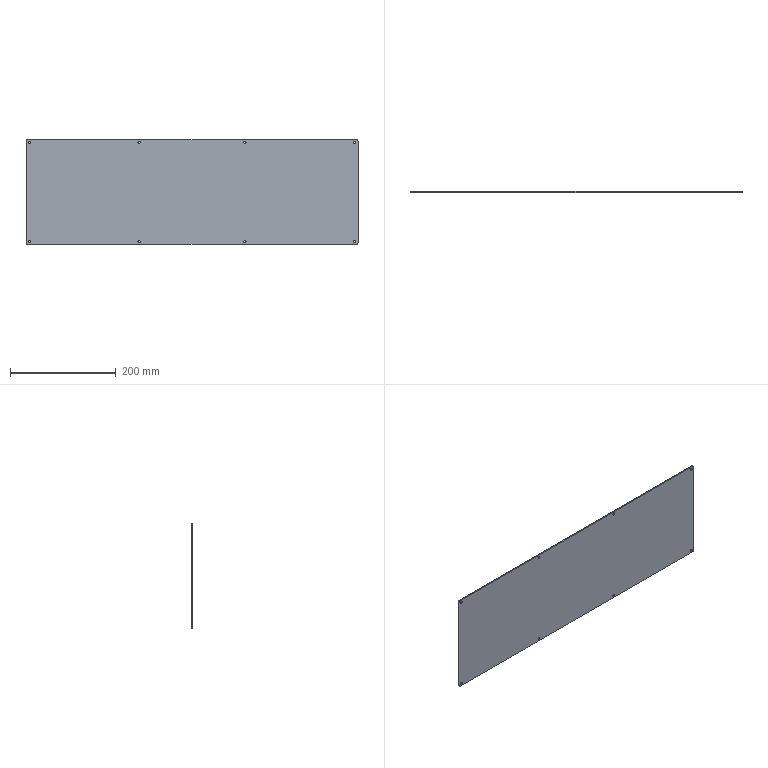Part | SolidWorks | features BaseBody 1 | 1 solid | 26 faces | box 628 x 2 x 198 mm | volume 248418 mm3 | cylinder 20 | plane 6 | commonest cylinder face diameters 4.5 x16 6 x4
STEP:
#1=CARTESIAN_POINT('',(307.5,0.,91.75));
#2=VERTEX_POINT('',#1);
#3=CARTESIAN_POINT('',(307.5,2.,91.75));
#4=VERTEX_POINT('',#3);
#5=CARTESIAN_POINT('',(307.5,-0.001,91.75));
#6=DIRECTION('',(0.,1.,0.));
#7=VECTOR('',#6,1000.);
#8=LINE('',#5,#7);
#9=EDGE_CURVE('',#2,#4,#8,.T.);
#10=ORIENTED_EDGE('',*,*,#9,.F.);
#11=CARTESIAN_POINT('',(307.5,0.,96.25));
#12=VERTEX_POINT('',#11);
#13=CARTESIAN_POINT('',(307.5,0.,94.));
#14=DIRECTION('',(0.,-1.,0.));
#15=DIRECTION('',(0.,0.,1.));
#16=AXIS2_PLACEMENT_3D('',#13,#14,#15);
#17=CIRCLE('',#16,2.25);
#18=EDGE_CURVE('',#2,#12,#17,.T.);
#19=ORIENTED_EDGE('',*,*,#18,.T.);
#20=CARTESIAN_POINT('',(307.5,2.,96.25));
#21=VERTEX_POINT('',#20);
#22=CARTESIAN_POINT('',(307.5,-0.001,96.25));
#23=DIRECTION('',(0.,1.,0.));
#24=VECTOR('',#23,1000.);
#25=LINE('',#22,#24);
#26=EDGE_CURVE('',#12,#21,#25,.T.);
#27=ORIENTED_EDGE('',*,*,#26,.T.);
#28=CARTESIAN_POINT('',(307.5,2.,94.));
#29=DIRECTION('',(0.,1.,0.));
#30=DIRECTION('',(0.,0.,1.));
#31=AXIS2_PLACEMENT_3D('',#28,#29,#30);
#32=CIRCLE('',#31,2.25);
#33=EDGE_CURVE('',#21,#4,#32,.T.);
#34=ORIENTED_EDGE('',*,*,#33,.T.);
#35=EDGE_LOOP('',(#10,#19,#27,#34));
#36=FACE_OUTER_BOUND('',#35,.T.);
#37=CARTESIAN_POINT('',(307.5,-0.001,94.));
#38=DIRECTION('',(0.,1.,0.));
#39=DIRECTION('',(0.,0.,1.));
#40=AXIS2_PLACEMENT_3D('',#37,#38,#39);
#41=CYLINDRICAL_SURFACE('',#40,2.25);
#42=ADVANCED_FACE('',(#36),#41,.F.);
#43=CARTESIAN_POINT('',(-307.5,0.,91.75));
#44=VERTEX_POINT('',#43);
#45=CARTESIAN_POINT('',(-307.5,2.,91.75));
#46=VERTEX_POINT('',#45);
#47=CARTESIAN_POINT('',(-307.5,-0.001,91.75));
#48=DIRECTION('',(0.,1.,0.));
#49=VECTOR('',#48,1000.);
#50=LINE('',#47,#49);
#51=EDGE_CURVE('',#44,#46,#50,.T.);
#52=ORIENTED_EDGE('',*,*,#51,.F.);
#53=CARTESIAN_POINT('',(-307.5,0.,96.25));
#54=VERTEX_POINT('',#53);
#55=CARTESIAN_POINT('',(-307.5,0.,94.));
#56=DIRECTION('',(0.,-1.,0.));
#57=DIRECTION('',(0.,0.,1.));
#58=AXIS2_PLACEMENT_3D('',#55,#56,#57);
#59=CIRCLE('',#58,2.25);
#60=EDGE_CURVE('',#44,#54,#59,.T.);
#61=ORIENTED_EDGE('',*,*,#60,.T.);
#62=CARTESIAN_POINT('',(-307.5,2.,96.25));
#63=VERTEX_POINT('',#62);
#64=CARTESIAN_POINT('',(-307.5,-0.001,96.25));
#65=DIRECTION('',(0.,1.,0.));
#66=VECTOR('',#65,1000.);
#67=LINE('',#64,#66);
#68=EDGE_CURVE('',#54,#63,#67,.T.);
#69=ORIENTED_EDGE('',*,*,#68,.T.);
#70=CARTESIAN_POINT('',(-307.5,2.,94.));
#71=DIRECTION('',(0.,1.,0.));
#72=DIRECTION('',(0.,0.,-1.));
#73=AXIS2_PLACEMENT_3D('',#70,#71,#72);
#74=CIRCLE('',#73,2.25);
#75=EDGE_CURVE('',#63,#46,#74,.T.);
#76=ORIENTED_EDGE('',*,*,#75,.T.);
#77=EDGE_LOOP('',(#52,#61,#69,#76));
#78=FACE_OUTER_BOUND('',#77,.T.);
#79=CARTESIAN_POINT('',(-307.5,-0.001,94.));
#80=DIRECTION('',(0.,1.,0.));
#81=DIRECTION('',(0.,0.,1.));
#82=AXIS2_PLACEMENT_3D('',#79,#80,#81);
#83=CYLINDRICAL_SURFACE('',#82,2.25);
#84=ADVANCED_FACE('',(#78),#83,.F.);
#85=CARTESIAN_POINT('',(-100.,0.,91.75));
#86=VERTEX_POINT('',#85);
#87=CARTESIAN_POINT('',(-100.,2.,91.75));
#88=VERTEX_POINT('',#87);
#89=CARTESIAN_POINT('',(-100.,-0.001,91.75));
#90=DIRECTION('',(0.,1.,0.));
#91=VECTOR('',#90,1000.);
#92=LINE('',#89,#91);
#93=EDGE_CURVE('',#86,#88,#92,.T.);
#94=ORIENTED_EDGE('',*,*,#93,.F.);
#95=CARTESIAN_POINT('',(-100.,0.,96.25));
#96=VERTEX_POINT('',#95);
#97=CARTESIAN_POINT('',(-100.,0.,94.));
#98=DIRECTION('',(0.,-1.,0.));
#99=DIRECTION('',(0.,0.,1.));
#100=AXIS2_PLACEMENT_3D('',#97,#98,#99);
#101=CIRCLE('',#100,2.25);
#102=EDGE_CURVE('',#86,#96,#101,.T.);
#103=ORIENTED_EDGE('',*,*,#102,.T.);
#104=CARTESIAN_POINT('',(-100.,2.,96.25));
#105=VERTEX_POINT('',#104);
#106=CARTESIAN_POINT('',(-100.,-0.001,96.25));
#107=DIRECTION('',(0.,1.,0.));
#108=VECTOR('',#107,1000.);
#109=LINE('',#106,#108);
#110=EDGE_CURVE('',#96,#105,#109,.T.);
#111=ORIENTED_EDGE('',*,*,#110,.T.);
#112=CARTESIAN_POINT('',(-100.,2.,94.));
#113=DIRECTION('',(0.,1.,0.));
#114=DIRECTION('',(0.,0.,-1.));
#115=AXIS2_PLACEMENT_3D('',#112,#113,#114);
#116=CIRCLE('',#115,2.25);
#117=EDGE_CURVE('',#105,#88,#116,.T.);
#118=ORIENTED_EDGE('',*,*,#117,.T.);
#119=EDGE_LOOP('',(#94,#103,#111,#118));
#120=FACE_OUTER_BOUND('',#119,.T.);
#121=CARTESIAN_POINT('',(-100.,-0.001,94.));
#122=DIRECTION('',(0.,1.,0.));
#123=DIRECTION('',(0.,0.,1.));
#124=AXIS2_PLACEMENT_3D('',#121,#122,#123);
#125=CYLINDRICAL_SURFACE('',#124,2.25);
#126=ADVANCED_FACE('',(#120),#125,.F.);
#127=CARTESIAN_POINT('',(-100.,0.,-96.25));
#128=VERTEX_POINT('',#127);
#129=CARTESIAN_POINT('',(-100.,2.,-96.25));
#130=VERTEX_POINT('',#129);
#131=CARTESIAN_POINT('',(-100.,-0.001,-96.25));
#132=DIRECTION('',(0.,1.,0.));
#133=VECTOR('',#132,1000.);
#134=LINE('',#131,#133);
#135=EDGE_CURVE('',#128,#130,#134,.T.);
#136=ORIENTED_EDGE('',*,*,#135,.F.);
#137=CARTESIAN_POINT('',(-100.,0.,-91.75));
#138=VERTEX_POINT('',#137);
#139=CARTESIAN_POINT('',(-100.,0.,-94.));
#140=DIRECTION('',(0.,-1.,0.));
#141=DIRECTION('',(0.,0.,1.));
#142=AXIS2_PLACEMENT_3D('',#139,#140,#141);
#143=CIRCLE('',#142,2.25);
#144=EDGE_CURVE('',#128,#138,#143,.T.);
#145=ORIENTED_EDGE('',*,*,#144,.T.);
#146=CARTESIAN_POINT('',(-100.,2.,-91.75));
#147=VERTEX_POINT('',#146);
#148=CARTESIAN_POINT('',(-100.,-0.001,-91.75));
#149=DIRECTION('',(0.,1.,0.));
#150=VECTOR('',#149,1000.);
#151=LINE('',#148,#150);
#152=EDGE_CURVE('',#138,#147,#151,.T.);
#153=ORIENTED_EDGE('',*,*,#152,.T.);
#154=CARTESIAN_POINT('',(-100.,2.,-94.));
#155=DIRECTION('',(0.,1.,0.));
#156=DIRECTION('',(0.,0.,1.));
#157=AXIS2_PLACEMENT_3D('',#154,#155,#156);
#158=CIRCLE('',#157,2.25);
#159=EDGE_CURVE('',#147,#130,#158,.T.);
#160=ORIENTED_EDGE('',*,*,#159,.T.);
#161=EDGE_LOOP('',(#136,#145,#153,#160));
#162=FACE_OUTER_BOUND('',#161,.T.);
#163=CARTESIAN_POINT('',(-100.,-0.001,-94.));
#164=DIRECTION('',(0.,1.,0.));
#165=DIRECTION('',(0.,0.,1.));
#166=AXIS2_PLACEMENT_3D('',#163,#164,#165);
#167=CYLINDRICAL_SURFACE('',#166,2.25);
#168=ADVANCED_FACE('',(#162),#167,.F.);
#169=CARTESIAN_POINT('',(100.,0.,91.75));
#170=VERTEX_POINT('',#169);
#171=CARTESIAN_POINT('',(100.,2.,91.75));
#172=VERTEX_POINT('',#171);
#173=CARTESIAN_POINT('',(100.,-0.001,91.75));
#174=DIRECTION('',(0.,1.,0.));
#175=VECTOR('',#174,1000.);
#176=LINE('',#173,#175);
#177=EDGE_CURVE('',#170,#172,#176,.T.);
#178=ORIENTED_EDGE('',*,*,#177,.F.);
#179=CARTESIAN_POINT('',(100.,0.,96.25));
#180=VERTEX_POINT('',#179);
#181=CARTESIAN_POINT('',(100.,0.,94.));
#182=DIRECTION('',(0.,-1.,0.));
#183=DIRECTION('',(0.,0.,1.));
#184=AXIS2_PLACEMENT_3D('',#181,#182,#183);
#185=CIRCLE('',#184,2.25);
#186=EDGE_CURVE('',#170,#180,#185,.T.);
#187=ORIENTED_EDGE('',*,*,#186,.T.);
#188=CARTESIAN_POINT('',(100.,2.,96.25));
#189=VERTEX_POINT('',#188);
#190=CARTESIAN_POINT('',(100.,-0.001,96.25));
#191=DIRECTION('',(0.,1.,0.));
#192=VECTOR('',#191,1000.);
#193=LINE('',#190,#192);
#194=EDGE_CURVE('',#180,#189,#193,.T.);
#195=ORIENTED_EDGE('',*,*,#194,.T.);
#196=CARTESIAN_POINT('',(100.,2.,94.));
#197=DIRECTION('',(0.,1.,0.));
#198=DIRECTION('',(0.,0.,1.));
#199=AXIS2_PLACEMENT_3D('',#196,#197,#198);
#200=CIRCLE('',#199,2.25);
#201=EDGE_CURVE('',#189,#172,#200,.T.);
#202=ORIENTED_EDGE('',*,*,#201,.T.);
#203=EDGE_LOOP('',(#178,#187,#195,#202));
#204=FACE_OUTER_BOUND('',#203,.T.);
#205=CARTESIAN_POINT('',(100.,-0.001,94.));
#206=DIRECTION('',(0.,1.,0.));
#207=DIRECTION('',(0.,0.,1.));
#208=AXIS2_PLACEMENT_3D('',#205,#206,#207);
#209=CYLINDRICAL_SURFACE('',#208,2.25);
#210=ADVANCED_FACE('',(#204),#209,.F.);
#211=CARTESIAN_POINT('',(100.,0.,-96.25));
#212=VERTEX_POINT('',#211);
#213=CARTESIAN_POINT('',(100.,2.,-96.25));
#214=VERTEX_POINT('',#213);
#215=CARTESIAN_POINT('',(100.,-0.001,-96.25));
#216=DIRECTION('',(0.,1.,0.));
#217=VECTOR('',#216,1000.);
#218=LINE('',#215,#217);
#219=EDGE_CURVE('',#212,#214,#218,.T.);
#220=ORIENTED_EDGE('',*,*,#219,.F.);
#221=CARTESIAN_POINT('',(100.,0.,-91.75));
#222=VERTEX_POINT('',#221);
#223=CARTESIAN_POINT('',(100.,0.,-94.));
#224=DIRECTION('',(0.,-1.,0.));
#225=DIRECTION('',(0.,0.,1.));
#226=AXIS2_PLACEMENT_3D('',#223,#224,#225);
#227=CIRCLE('',#226,2.25);
#228=EDGE_CURVE('',#212,#222,#227,.T.);
#229=ORIENTED_EDGE('',*,*,#228,.T.);
#230=CARTESIAN_POINT('',(100.,2.,-91.75));
#231=VERTEX_POINT('',#230);
#232=CARTESIAN_POINT('',(100.,-0.001,-91.75));
#233=DIRECTION('',(0.,1.,0.));
#234=VECTOR('',#233,1000.);
#235=LINE('',#232,#234);
#236=EDGE_CURVE('',#222,#231,#235,.T.);
#237=ORIENTED_EDGE('',*,*,#236,.T.);
#238=CARTESIAN_POINT('',(100.,2.,-94.));
#239=DIRECTION('',(0.,1.,0.));
#240=DIRECTION('',(0.,0.,-1.));
#241=AXIS2_PLACEMENT_3D('',#238,#239,#240);
#242=CIRCLE('',#241,2.25);
#243=EDGE_CURVE('',#231,#214,#242,.T.);
#244=ORIENTED_EDGE('',*,*,#243,.T.);
#245=EDGE_LOOP('',(#220,#229,#237,#244));
#246=FACE_OUTER_BOUND('',#245,.T.);
#247=CARTESIAN_POINT('',(100.,-0.001,-94.));
#248=DIRECTION('',(0.,1.,0.));
#249=DIRECTION('',(0.,0.,1.));
#250=AXIS2_PLACEMENT_3D('',#247,#248,#249);
#251=CYLINDRICAL_SURFACE('',#250,2.25);
#252=ADVANCED_FACE('',(#246),#251,.F.);
#253=CARTESIAN_POINT('',(307.5,0.,-96.25));
#254=VERTEX_POINT('',#253);
#255=CARTESIAN_POINT('',(307.5,2.,-96.25));
#256=VERTEX_POINT('',#255);
#257=CARTESIAN_POINT('',(307.5,-0.001,-96.25));
#258=DIRECTION('',(0.,1.,0.));
#259=VECTOR('',#258,1000.);
#260=LINE('',#257,#259);
#261=EDGE_CURVE('',#254,#256,#260,.T.);
#262=ORIENTED_EDGE('',*,*,#261,.F.);
#263=CARTESIAN_POINT('',(307.5,0.,-91.75));
#264=VERTEX_POINT('',#263);
#265=CARTESIAN_POINT('',(307.5,0.,-94.));
#266=DIRECTION('',(0.,-1.,0.));
#267=DIRECTION('',(0.,0.,1.));
#268=AXIS2_PLACEMENT_3D('',#265,#266,#267);
#269=CIRCLE('',#268,2.25);
#270=EDGE_CURVE('',#254,#264,#269,.T.);
#271=ORIENTED_EDGE('',*,*,#270,.T.);
#272=CARTESIAN_POINT('',(307.5,2.,-91.75));
#273=VERTEX_POINT('',#272);
#274=CARTESIAN_POINT('',(307.5,-0.001,-91.75));
#275=DIRECTION('',(0.,1.,0.));
#276=VECTOR('',#275,1000.);
#277=LINE('',#274,#276);
#278=EDGE_CURVE('',#264,#273,#277,.T.);
#279=ORIENTED_EDGE('',*,*,#278,.T.);
#280=CARTESIAN_POINT('',(307.5,2.,-94.));
#281=DIRECTION('',(0.,1.,0.));
#282=DIRECTION('',(0.,0.,-1.));
#283=AXIS2_PLACEMENT_3D('',#280,#281,#282);
#284=CIRCLE('',#283,2.25);
#285=EDGE_CURVE('',#273,#256,#284,.T.);
#286=ORIENTED_EDGE('',*,*,#285,.T.);
#287=EDGE_LOOP('',(#262,#271,#279,#286));
#288=FACE_OUTER_BOUND('',#287,.T.);
#289=CARTESIAN_POINT('',(307.5,-0.001,-94.));
#290=DIRECTION('',(0.,1.,0.));
#291=DIRECTION('',(0.,0.,1.));
#292=AXIS2_PLACEMENT_3D('',#289,#290,#291);
#293=CYLINDRICAL_SURFACE('',#292,2.25);
#294=ADVANCED_FACE('',(#288),#293,.F.);
#295=CARTESIAN_POINT('',(-307.5,0.,-96.25));
#296=VERTEX_POINT('',#295);
#297=CARTESIAN_POINT('',(-307.5,2.,-96.25));
#298=VERTEX_POINT('',#297);
#299=CARTESIAN_POINT('',(-307.5,-0.001,-96.25));
#300=DIRECTION('',(0.,1.,0.));
#301=VECTOR('',#300,1000.);
#302=LINE('',#299,#301);
#303=EDGE_CURVE('',#296,#298,#302,.T.);
#304=ORIENTED_EDGE('',*,*,#303,.F.);
#305=CARTESIAN_POINT('',(-307.5,0.,-91.75));
#306=VERTEX_POINT('',#305);
#307=CARTESIAN_POINT('',(-307.5,0.,-94.));
#308=DIRECTION('',(0.,-1.,0.));
#309=DIRECTION('',(0.,0.,1.));
#310=AXIS2_PLACEMENT_3D('',#307,#308,#309);
#311=CIRCLE('',#310,2.25);
#312=EDGE_CURVE('',#296,#306,#311,.T.);
#313=ORIENTED_EDGE('',*,*,#312,.T.);
#314=CARTESIAN_POINT('',(-307.5,2.,-91.75));
#315=VERTEX_POINT('',#314);
#316=CARTESIAN_POINT('',(-307.5,-0.001,-91.75));
#317=DIRECTION('',(0.,1.,0.));
#318=VECTOR('',#317,1000.);
#319=LINE('',#316,#318);
#320=EDGE_CURVE('',#306,#315,#319,.T.);
#321=ORIENTED_EDGE('',*,*,#320,.T.);
#322=CARTESIAN_POINT('',(-307.5,2.,-94.));
#323=DIRECTION('',(0.,1.,0.));
#324=DIRECTION('',(0.,0.,1.));
#325=AXIS2_PLACEMENT_3D('',#322,#323,#324);
#326=CIRCLE('',#325,2.25);
#327=EDGE_CURVE('',#315,#298,#326,.T.);
#328=ORIENTED_EDGE('',*,*,#327,.T.);
#329=EDGE_LOOP('',(#304,#313,#321,#328));
#330=FACE_OUTER_BOUND('',#329,.T.);
#331=CARTESIAN_POINT('',(-307.5,-0.001,-94.));
#332=DIRECTION('',(0.,1.,0.));
#333=DIRECTION('',(0.,0.,1.));
#334=AXIS2_PLACEMENT_3D('',#331,#332,#333);
#335=CYLINDRICAL_SURFACE('',#334,2.25);
#336=ADVANCED_FACE('',(#330),#335,.F.);
#337=CARTESIAN_POINT('',(311.,2.,99.));
#338=VERTEX_POINT('',#337);
#339=CARTESIAN_POINT('',(314.,2.,96.));
#340=VERTEX_POINT('',#339);
#341=CARTESIAN_POINT('',(311.,2.,96.));
#342=DIRECTION('',(0.,1.,0.));
#343=DIRECTION('',(0.,0.,1.));
#344=AXIS2_PLACEMENT_3D('',#341,#342,#343);
#345=CIRCLE('',#344,3.);
#346=EDGE_CURVE('',#338,#340,#345,.T.);
#347=ORIENTED_EDGE('',*,*,#346,.F.);
#348=CARTESIAN_POINT('',(311.,0.,99.));
#349=VERTEX_POINT('',#348);
#350=CARTESIAN_POINT('',(311.,2.,99.));
#351=DIRECTION('',(0.,1.,0.));
#352=VECTOR('',#351,1000.);
#353=LINE('',#350,#352);
#354=EDGE_CURVE('',#349,#338,#353,.T.);
#355=ORIENTED_EDGE('',*,*,#354,.F.);
#356=CARTESIAN_POINT('',(314.,0.,96.));
#357=VERTEX_POINT('',#356);
#358=CARTESIAN_POINT('',(311.,0.,96.));
#359=DIRECTION('',(0.,-1.,0.));
#360=DIRECTION('',(0.,0.,1.));
#361=AXIS2_PLACEMENT_3D('',#358,#359,#360);
#362=CIRCLE('',#361,3.);
#363=EDGE_CURVE('',#357,#349,#362,.T.);
#364=ORIENTED_EDGE('',*,*,#363,.F.);
#365=CARTESIAN_POINT('',(314.,2.,96.));
#366=DIRECTION('',(0.,-1.,0.));
#367=VECTOR('',#366,1000.);
#368=LINE('',#365,#367);
#369=EDGE_CURVE('',#340,#357,#368,.T.);
#370=ORIENTED_EDGE('',*,*,#369,.F.);
#371=EDGE_LOOP('',(#347,#355,#364,#370));
#372=FACE_OUTER_BOUND('',#371,.T.);
#373=CARTESIAN_POINT('',(311.,2.,96.));
#374=DIRECTION('',(0.,-1.,0.));
#375=DIRECTION('',(0.,0.,-1.));
#376=AXIS2_PLACEMENT_3D('',#373,#374,#375);
#377=CYLINDRICAL_SURFACE('',#376,3.);
#378=ADVANCED_FACE('',(#372),#377,.T.);
#379=CARTESIAN_POINT('',(-314.,2.,96.));
#380=VERTEX_POINT('',#379);
#381=CARTESIAN_POINT('',(-311.,2.,99.));
#382=VERTEX_POINT('',#381);
#383=CARTESIAN_POINT('',(-311.,2.,96.));
#384=DIRECTION('',(0.,1.,0.));
#385=DIRECTION('',(0.,0.,1.));
#386=AXIS2_PLACEMENT_3D('',#383,#384,#385);
#387=CIRCLE('',#386,3.);
#388=EDGE_CURVE('',#380,#382,#387,.T.);
#389=ORIENTED_EDGE('',*,*,#388,.F.);
#390=CARTESIAN_POINT('',(-314.,0.,96.));
#391=VERTEX_POINT('',#390);
#392=CARTESIAN_POINT('',(-314.,2.,96.));
#393=DIRECTION('',(0.,1.,0.));
#394=VECTOR('',#393,1000.);
#395=LINE('',#392,#394);
#396=EDGE_CURVE('',#391,#380,#395,.T.);
#397=ORIENTED_EDGE('',*,*,#396,.F.);
#398=CARTESIAN_POINT('',(-311.,0.,99.));
#399=VERTEX_POINT('',#398);
#400=CARTESIAN_POINT('',(-311.,0.,96.));
#401=DIRECTION('',(0.,-1.,0.));
#402=DIRECTION('',(0.,0.,1.));
#403=AXIS2_PLACEMENT_3D('',#400,#401,#402);
#404=CIRCLE('',#403,3.);
#405=EDGE_CURVE('',#399,#391,#404,.T.);
#406=ORIENTED_EDGE('',*,*,#405,.F.);
#407=CARTESIAN_POINT('',(-311.,2.,99.));
#408=DIRECTION('',(0.,-1.,0.));
#409=VECTOR('',#408,1000.);
#410=LINE('',#407,#409);
#411=EDGE_CURVE('',#382,#399,#410,.T.);
#412=ORIENTED_EDGE('',*,*,#411,.F.);
#413=EDGE_LOOP('',(#389,#397,#406,#412));
#414=FACE_OUTER_BOUND('',#413,.T.);
#415=CARTESIAN_POINT('',(-311.,2.,96.));
#416=DIRECTION('',(0.,-1.,0.));
#417=DIRECTION('',(0.,0.,-1.));
#418=AXIS2_PLACEMENT_3D('',#415,#416,#417);
#419=CYLINDRICAL_SURFACE('',#418,3.);
#420=ADVANCED_FACE('',(#414),#419,.T.);
#421=CARTESIAN_POINT('',(314.,2.,-96.));
#422=VERTEX_POINT('',#421);
#423=CARTESIAN_POINT('',(311.,2.,-99.));
#424=VERTEX_POINT('',#423);
#425=CARTESIAN_POINT('',(311.,2.,-96.));
#426=DIRECTION('',(0.,1.,0.));
#427=DIRECTION('',(0.,0.,1.));
#428=AXIS2_PLACEMENT_3D('',#425,#426,#427);
#429=CIRCLE('',#428,3.);
#430=EDGE_CURVE('',#422,#424,#429,.T.);
#431=ORIENTED_EDGE('',*,*,#430,.F.);
#432=CARTESIAN_POINT('',(314.,0.,-96.));
#433=VERTEX_POINT('',#432);
#434=CARTESIAN_POINT('',(314.,2.,-96.));
#435=DIRECTION('',(0.,1.,0.));
#436=VECTOR('',#435,1000.);
#437=LINE('',#434,#436);
#438=EDGE_CURVE('',#433,#422,#437,.T.);
#439=ORIENTED_EDGE('',*,*,#438,.F.);
#440=CARTESIAN_POINT('',(311.,0.,-99.));
#441=VERTEX_POINT('',#440);
#442=CARTESIAN_POINT('',(311.,0.,-96.));
#443=DIRECTION('',(0.,-1.,0.));
#444=DIRECTION('',(0.,0.,1.));
#445=AXIS2_PLACEMENT_3D('',#442,#443,#444);
#446=CIRCLE('',#445,3.);
#447=EDGE_CURVE('',#441,#433,#446,.T.);
#448=ORIENTED_EDGE('',*,*,#447,.F.);
#449=CARTESIAN_POINT('',(311.,2.,-99.));
#450=DIRECTION('',(0.,-1.,0.));
#451=VECTOR('',#450,1000.);
#452=LINE('',#449,#451);
#453=EDGE_CURVE('',#424,#441,#452,.T.);
#454=ORIENTED_EDGE('',*,*,#453,.F.);
#455=EDGE_LOOP('',(#431,#439,#448,#454));
#456=FACE_OUTER_BOUND('',#455,.T.);
#457=CARTESIAN_POINT('',(311.,2.,-96.));
#458=DIRECTION('',(0.,-1.,0.));
#459=DIRECTION('',(0.,0.,-1.));
#460=AXIS2_PLACEMENT_3D('',#457,#458,#459);
#461=CYLINDRICAL_SURFACE('',#460,3.);
#462=ADVANCED_FACE('',(#456),#461,.T.);
#463=CARTESIAN_POINT('',(-311.,2.,-99.));
#464=VERTEX_POINT('',#463);
#465=CARTESIAN_POINT('',(-314.,2.,-96.));
#466=VERTEX_POINT('',#465);
#467=CARTESIAN_POINT('',(-311.,2.,-96.));
#468=DIRECTION('',(0.,1.,0.));
#469=DIRECTION('',(0.,0.,1.));
#470=AXIS2_PLACEMENT_3D('',#467,#468,#469);
#471=CIRCLE('',#470,3.);
#472=EDGE_CURVE('',#464,#466,#471,.T.);
#473=ORIENTED_EDGE('',*,*,#472,.F.);
#474=CARTESIAN_POINT('',(-311.,0.,-99.));
#475=VERTEX_POINT('',#474);
#476=CARTESIAN_POINT('',(-311.,2.,-99.));
#477=DIRECTION('',(0.,1.,0.));
#478=VECTOR('',#477,1000.);
#479=LINE('',#476,#478);
#480=EDGE_CURVE('',#475,#464,#479,.T.);
#481=ORIENTED_EDGE('',*,*,#480,.F.);
#482=CARTESIAN_POINT('',(-314.,0.,-96.));
#483=VERTEX_POINT('',#482);
#484=CARTESIAN_POINT('',(-311.,0.,-96.));
#485=DIRECTION('',(0.,-1.,0.));
#486=DIRECTION('',(0.,0.,1.));
#487=AXIS2_PLACEMENT_3D('',#484,#485,#486);
#488=CIRCLE('',#487,3.);
#489=EDGE_CURVE('',#483,#475,#488,.T.);
#490=ORIENTED_EDGE('',*,*,#489,.F.);
#491=CARTESIAN_POINT('',(-314.,2.,-96.));
#492=DIRECTION('',(0.,-1.,0.));
#493=VECTOR('',#492,1000.);
#494=LINE('',#491,#493);
#495=EDGE_CURVE('',#466,#483,#494,.T.);
#496=ORIENTED_EDGE('',*,*,#495,.F.);
#497=EDGE_LOOP('',(#473,#481,#490,#496));
#498=FACE_OUTER_BOUND('',#497,.T.);
#499=CARTESIAN_POINT('',(-311.,2.,-96.));
#500=DIRECTION('',(0.,-1.,0.));
#501=DIRECTION('',(0.,0.,-1.));
#502=AXIS2_PLACEMENT_3D('',#499,#500,#501);
#503=CYLINDRICAL_SURFACE('',#502,3.);
#504=ADVANCED_FACE('',(#498),#503,.T.);
#505=CARTESIAN_POINT('',(-307.5,0.,-94.));
#506=DIRECTION('',(0.,-1.,0.));
#507=DIRECTION('',(0.,0.,1.));
#508=AXIS2_PLACEMENT_3D('',#505,#506,#507);
#509=CIRCLE('',#508,2.25);
#510=EDGE_CURVE('',#306,#296,#509,.T.);
#511=ORIENTED_EDGE('',*,*,#510,.F.);
#512=ORIENTED_EDGE('',*,*,#312,.F.);
#513=EDGE_LOOP('',(#511,#512));
#514=FACE_BOUND('',#513,.T.);
#515=CARTESIAN_POINT('',(307.5,0.,-94.));
#516=DIRECTION('',(0.,-1.,0.));
#517=DIRECTION('',(0.,0.,1.));
#518=AXIS2_PLACEMENT_3D('',#515,#516,#517);
#519=CIRCLE('',#518,2.25);
#520=EDGE_CURVE('',#264,#254,#519,.T.);
#521=ORIENTED_EDGE('',*,*,#520,.F.);
#522=ORIENTED_EDGE('',*,*,#270,.F.);
#523=EDGE_LOOP('',(#521,#522));
#524=FACE_BOUND('',#523,.T.);
#525=CARTESIAN_POINT('',(100.,0.,-94.));
#526=DIRECTION('',(0.,-1.,0.));
#527=DIRECTION('',(0.,0.,1.));
#528=AXIS2_PLACEMENT_3D('',#525,#526,#527);
#529=CIRCLE('',#528,2.25);
#530=EDGE_CURVE('',#222,#212,#529,.T.);
#531=ORIENTED_EDGE('',*,*,#530,.F.);
#532=ORIENTED_EDGE('',*,*,#228,.F.);
#533=EDGE_LOOP('',(#531,#532));
#534=FACE_BOUND('',#533,.T.);
#535=CARTESIAN_POINT('',(100.,0.,94.));
#536=DIRECTION('',(0.,-1.,0.));
#537=DIRECTION('',(0.,0.,1.));
#538=AXIS2_PLACEMENT_3D('',#535,#536,#537);
#539=CIRCLE('',#538,2.25);
#540=EDGE_CURVE('',#180,#170,#539,.T.);
#541=ORIENTED_EDGE('',*,*,#540,.F.);
#542=ORIENTED_EDGE('',*,*,#186,.F.);
#543=EDGE_LOOP('',(#541,#542));
#544=FACE_BOUND('',#543,.T.);
#545=CARTESIAN_POINT('',(-100.,0.,-94.));
#546=DIRECTION('',(0.,-1.,0.));
#547=DIRECTION('',(0.,0.,1.));
#548=AXIS2_PLACEMENT_3D('',#545,#546,#547);
#549=CIRCLE('',#548,2.25);
#550=EDGE_CURVE('',#138,#128,#549,.T.);
#551=ORIENTED_EDGE('',*,*,#550,.F.);
#552=ORIENTED_EDGE('',*,*,#144,.F.);
#553=EDGE_LOOP('',(#551,#552));
#554=FACE_BOUND('',#553,.T.);
#555=CARTESIAN_POINT('',(-100.,0.,94.));
#556=DIRECTION('',(0.,-1.,0.));
#557=DIRECTION('',(0.,0.,1.));
#558=AXIS2_PLACEMENT_3D('',#555,#556,#557);
#559=CIRCLE('',#558,2.25);
#560=EDGE_CURVE('',#96,#86,#559,.T.);
#561=ORIENTED_EDGE('',*,*,#560,.F.);
#562=ORIENTED_EDGE('',*,*,#102,.F.);
#563=EDGE_LOOP('',(#561,#562));
#564=FACE_BOUND('',#563,.T.);
#565=CARTESIAN_POINT('',(-307.5,0.,94.));
#566=DIRECTION('',(0.,-1.,0.));
#567=DIRECTION('',(0.,0.,1.));
#568=AXIS2_PLACEMENT_3D('',#565,#566,#567);
#569=CIRCLE('',#568,2.25);
#570=EDGE_CURVE('',#54,#44,#569,.T.);
#571=ORIENTED_EDGE('',*,*,#570,.F.);
#572=ORIENTED_EDGE('',*,*,#60,.F.);
#573=EDGE_LOOP('',(#571,#572));
#574=FACE_BOUND('',#573,.T.);
#575=CARTESIAN_POINT('',(307.5,0.,94.));
#576=DIRECTION('',(0.,-1.,0.));
#577=DIRECTION('',(0.,0.,1.));
#578=AXIS2_PLACEMENT_3D('',#575,#576,#577);
#579=CIRCLE('',#578,2.25);
#580=EDGE_CURVE('',#12,#2,#579,.T.);
#581=ORIENTED_EDGE('',*,*,#580,.F.);
#582=ORIENTED_EDGE('',*,*,#18,.F.);
#583=EDGE_LOOP('',(#581,#582));
#584=FACE_BOUND('',#583,.T.);
#585=CARTESIAN_POINT('',(-314.,0.,99.));
#586=DIRECTION('',(0.,0.,1.));
#587=VECTOR('',#586,1000.);
#588=LINE('',#585,#587);
#589=EDGE_CURVE('',#483,#391,#588,.T.);
#590=ORIENTED_EDGE('',*,*,#589,.F.);
#591=ORIENTED_EDGE('',*,*,#489,.T.);
#592=CARTESIAN_POINT('',(314.,0.,-99.));
#593=DIRECTION('',(-1.,0.,0.));
#594=VECTOR('',#593,1000.);
#595=LINE('',#592,#594);
#596=EDGE_CURVE('',#441,#475,#595,.T.);
#597=ORIENTED_EDGE('',*,*,#596,.F.);
#598=ORIENTED_EDGE('',*,*,#447,.T.);
#599=CARTESIAN_POINT('',(314.,0.,99.));
#600=DIRECTION('',(0.,0.,-1.));
#601=VECTOR('',#600,1000.);
#602=LINE('',#599,#601);
#603=EDGE_CURVE('',#357,#433,#602,.T.);
#604=ORIENTED_EDGE('',*,*,#603,.F.);
#605=ORIENTED_EDGE('',*,*,#363,.T.);
#606=CARTESIAN_POINT('',(314.,0.,99.));
#607=DIRECTION('',(1.,0.,0.));
#608=VECTOR('',#607,1000.);
#609=LINE('',#606,#608);
#610=EDGE_CURVE('',#399,#349,#609,.T.);
#611=ORIENTED_EDGE('',*,*,#610,.F.);
#612=ORIENTED_EDGE('',*,*,#405,.T.);
#613=EDGE_LOOP('',(#590,#591,#597,#598,#604,#605,#611,#612));
#614=FACE_OUTER_BOUND('',#613,.T.);
#615=CARTESIAN_POINT('',(0.,0.,0.));
#616=DIRECTION('',(0.,1.,0.));
#617=DIRECTION('',(1.,0.,0.));
#618=AXIS2_PLACEMENT_3D('',#615,#616,#617);
#619=PLANE('',#618);
#620=ADVANCED_FACE('',(#514,#524,#534,#544,#554,#564,#574,#584,#614),#619,.F.);
#621=ORIENTED_EDGE('',*,*,#327,.F.);
#622=CARTESIAN_POINT('',(-307.5,2.,-94.));
#623=DIRECTION('',(0.,1.,0.));
#624=DIRECTION('',(0.,0.,1.));
#625=AXIS2_PLACEMENT_3D('',#622,#623,#624);
#626=CIRCLE('',#625,2.25);
#627=EDGE_CURVE('',#298,#315,#626,.T.);
#628=ORIENTED_EDGE('',*,*,#627,.F.);
#629=EDGE_LOOP('',(#621,#628));
#630=FACE_BOUND('',#629,.T.);
#631=ORIENTED_EDGE('',*,*,#285,.F.);
#632=CARTESIAN_POINT('',(307.5,2.,-94.));
#633=DIRECTION('',(0.,1.,0.));
#634=DIRECTION('',(0.,0.,-1.));
#635=AXIS2_PLACEMENT_3D('',#632,#633,#634);
#636=CIRCLE('',#635,2.25);
#637=EDGE_CURVE('',#256,#273,#636,.T.);
#638=ORIENTED_EDGE('',*,*,#637,.F.);
#639=EDGE_LOOP('',(#631,#638));
#640=FACE_BOUND('',#639,.T.);
#641=ORIENTED_EDGE('',*,*,#243,.F.);
#642=CARTESIAN_POINT('',(100.,2.,-94.));
#643=DIRECTION('',(0.,1.,0.));
#644=DIRECTION('',(0.,0.,-1.));
#645=AXIS2_PLACEMENT_3D('',#642,#643,#644);
#646=CIRCLE('',#645,2.25);
#647=EDGE_CURVE('',#214,#231,#646,.T.);
#648=ORIENTED_EDGE('',*,*,#647,.F.);
#649=EDGE_LOOP('',(#641,#648));
#650=FACE_BOUND('',#649,.T.);
#651=ORIENTED_EDGE('',*,*,#201,.F.);
#652=CARTESIAN_POINT('',(100.,2.,94.));
#653=DIRECTION('',(0.,1.,0.));
#654=DIRECTION('',(0.,0.,1.));
#655=AXIS2_PLACEMENT_3D('',#652,#653,#654);
#656=CIRCLE('',#655,2.25);
#657=EDGE_CURVE('',#172,#189,#656,.T.);
#658=ORIENTED_EDGE('',*,*,#657,.F.);
#659=EDGE_LOOP('',(#651,#658));
#660=FACE_BOUND('',#659,.T.);
#661=ORIENTED_EDGE('',*,*,#159,.F.);
#662=CARTESIAN_POINT('',(-100.,2.,-94.));
#663=DIRECTION('',(0.,1.,0.));
#664=DIRECTION('',(0.,0.,1.));
#665=AXIS2_PLACEMENT_3D('',#662,#663,#664);
#666=CIRCLE('',#665,2.25);
#667=EDGE_CURVE('',#130,#147,#666,.T.);
#668=ORIENTED_EDGE('',*,*,#667,.F.);
#669=EDGE_LOOP('',(#661,#668));
#670=FACE_BOUND('',#669,.T.);
#671=ORIENTED_EDGE('',*,*,#117,.F.);
#672=CARTESIAN_POINT('',(-100.,2.,94.));
#673=DIRECTION('',(0.,1.,0.));
#674=DIRECTION('',(0.,0.,-1.));
#675=AXIS2_PLACEMENT_3D('',#672,#673,#674);
#676=CIRCLE('',#675,2.25);
#677=EDGE_CURVE('',#88,#105,#676,.T.);
#678=ORIENTED_EDGE('',*,*,#677,.F.);
#679=EDGE_LOOP('',(#671,#678));
#680=FACE_BOUND('',#679,.T.);
#681=ORIENTED_EDGE('',*,*,#75,.F.);
#682=CARTESIAN_POINT('',(-307.5,2.,94.));
#683=DIRECTION('',(0.,1.,0.));
#684=DIRECTION('',(0.,0.,-1.));
#685=AXIS2_PLACEMENT_3D('',#682,#683,#684);
#686=CIRCLE('',#685,2.25);
#687=EDGE_CURVE('',#46,#63,#686,.T.);
#688=ORIENTED_EDGE('',*,*,#687,.F.);
#689=EDGE_LOOP('',(#681,#688));
#690=FACE_BOUND('',#689,.T.);
#691=ORIENTED_EDGE('',*,*,#33,.F.);
#692=CARTESIAN_POINT('',(307.5,2.,94.));
#693=DIRECTION('',(0.,1.,0.));
#694=DIRECTION('',(0.,0.,1.));
#695=AXIS2_PLACEMENT_3D('',#692,#693,#694);
#696=CIRCLE('',#695,2.25);
#697=EDGE_CURVE('',#4,#21,#696,.T.);
#698=ORIENTED_EDGE('',*,*,#697,.F.);
#699=EDGE_LOOP('',(#691,#698));
#700=FACE_BOUND('',#699,.T.);
#701=CARTESIAN_POINT('',(314.,2.,-99.));
#702=DIRECTION('',(-1.,0.,0.));
#703=VECTOR('',#702,1000.);
#704=LINE('',#701,#703);
#705=EDGE_CURVE('',#424,#464,#704,.T.);
#706=ORIENTED_EDGE('',*,*,#705,.T.);
#707=ORIENTED_EDGE('',*,*,#472,.T.);
#708=CARTESIAN_POINT('',(-314.,2.,99.));
#709=DIRECTION('',(0.,0.,1.));
#710=VECTOR('',#709,1000.);
#711=LINE('',#708,#710);
#712=EDGE_CURVE('',#466,#380,#711,.T.);
#713=ORIENTED_EDGE('',*,*,#712,.T.);
#714=ORIENTED_EDGE('',*,*,#388,.T.);
#715=CARTESIAN_POINT('',(314.,2.,99.));
#716=DIRECTION('',(1.,0.,0.));
#717=VECTOR('',#716,1000.);
#718=LINE('',#715,#717);
#719=EDGE_CURVE('',#382,#338,#718,.T.);
#720=ORIENTED_EDGE('',*,*,#719,.T.);
#721=ORIENTED_EDGE('',*,*,#346,.T.);
#722=CARTESIAN_POINT('',(314.,2.,99.));
#723=DIRECTION('',(0.,0.,-1.));
#724=VECTOR('',#723,1000.);
#725=LINE('',#722,#724);
#726=EDGE_CURVE('',#340,#422,#725,.T.);
#727=ORIENTED_EDGE('',*,*,#726,.T.);
#728=ORIENTED_EDGE('',*,*,#430,.T.);
#729=EDGE_LOOP('',(#706,#707,#713,#714,#720,#721,#727,#728));
#730=FACE_OUTER_BOUND('',#729,.T.);
#731=CARTESIAN_POINT('',(0.,2.,0.));
#732=DIRECTION('',(0.,1.,0.));
#733=DIRECTION('',(1.,0.,0.));
#734=AXIS2_PLACEMENT_3D('',#731,#732,#733);
#735=PLANE('',#734);
#736=ADVANCED_FACE('',(#630,#640,#650,#660,#670,#680,#690,#700,#730),#735,.T.);
#737=ORIENTED_EDGE('',*,*,#596,.T.);
#738=ORIENTED_EDGE('',*,*,#480,.T.);
#739=ORIENTED_EDGE('',*,*,#705,.F.);
#740=ORIENTED_EDGE('',*,*,#453,.T.);
#741=EDGE_LOOP('',(#737,#738,#739,#740));
#742=FACE_OUTER_BOUND('',#741,.T.);
#743=CARTESIAN_POINT('',(314.,2.,-99.));
#744=DIRECTION('',(0.,0.,1.));
#745=DIRECTION('',(1.,0.,0.));
#746=AXIS2_PLACEMENT_3D('',#743,#744,#745);
#747=PLANE('',#746);
#748=ADVANCED_FACE('',(#742),#747,.F.);
#749=ORIENTED_EDGE('',*,*,#603,.T.);
#750=ORIENTED_EDGE('',*,*,#438,.T.);
#751=ORIENTED_EDGE('',*,*,#726,.F.);
#752=ORIENTED_EDGE('',*,*,#369,.T.);
#753=EDGE_LOOP('',(#749,#750,#751,#752));
#754=FACE_OUTER_BOUND('',#753,.T.);
#755=CARTESIAN_POINT('',(314.,2.,99.));
#756=DIRECTION('',(-1.,0.,0.));
#757=DIRECTION('',(0.,0.,1.));
#758=AXIS2_PLACEMENT_3D('',#755,#756,#757);
#759=PLANE('',#758);
#760=ADVANCED_FACE('',(#754),#759,.F.);
#761=ORIENTED_EDGE('',*,*,#719,.F.);
#762=ORIENTED_EDGE('',*,*,#411,.T.);
#763=ORIENTED_EDGE('',*,*,#610,.T.);
#764=ORIENTED_EDGE('',*,*,#354,.T.);
#765=EDGE_LOOP('',(#761,#762,#763,#764));
#766=FACE_OUTER_BOUND('',#765,.T.);
#767=CARTESIAN_POINT('',(314.,2.,99.));
#768=DIRECTION('',(0.,0.,-1.));
#769=DIRECTION('',(-1.,0.,0.));
#770=AXIS2_PLACEMENT_3D('',#767,#768,#769);
#771=PLANE('',#770);
#772=ADVANCED_FACE('',(#766),#771,.F.);
#773=ORIENTED_EDGE('',*,*,#712,.F.);
#774=ORIENTED_EDGE('',*,*,#495,.T.);
#775=ORIENTED_EDGE('',*,*,#589,.T.);
#776=ORIENTED_EDGE('',*,*,#396,.T.);
#777=EDGE_LOOP('',(#773,#774,#775,#776));
#778=FACE_OUTER_BOUND('',#777,.T.);
#779=CARTESIAN_POINT('',(-314.,2.,99.));
#780=DIRECTION('',(1.,0.,0.));
#781=DIRECTION('',(0.,1.,0.));
#782=AXIS2_PLACEMENT_3D('',#779,#780,#781);
#783=PLANE('',#782);
#784=ADVANCED_FACE('',(#778),#783,.F.);
#785=ORIENTED_EDGE('',*,*,#510,.T.);
#786=ORIENTED_EDGE('',*,*,#303,.T.);
#787=ORIENTED_EDGE('',*,*,#627,.T.);
#788=ORIENTED_EDGE('',*,*,#320,.F.);
#789=EDGE_LOOP('',(#785,#786,#787,#788));
#790=FACE_OUTER_BOUND('',#789,.T.);
#791=CARTESIAN_POINT('',(-307.5,-0.001,-94.));
#792=DIRECTION('',(0.,1.,0.));
#793=DIRECTION('',(0.,0.,1.));
#794=AXIS2_PLACEMENT_3D('',#791,#792,#793);
#795=CYLINDRICAL_SURFACE('',#794,2.25);
#796=ADVANCED_FACE('',(#790),#795,.F.);
#797=ORIENTED_EDGE('',*,*,#520,.T.);
#798=ORIENTED_EDGE('',*,*,#261,.T.);
#799=ORIENTED_EDGE('',*,*,#637,.T.);
#800=ORIENTED_EDGE('',*,*,#278,.F.);
#801=EDGE_LOOP('',(#797,#798,#799,#800));
#802=FACE_OUTER_BOUND('',#801,.T.);
#803=CARTESIAN_POINT('',(307.5,-0.001,-94.));
#804=DIRECTION('',(0.,1.,0.));
#805=DIRECTION('',(0.,0.,1.));
#806=AXIS2_PLACEMENT_3D('',#803,#804,#805);
#807=CYLINDRICAL_SURFACE('',#806,2.25);
#808=ADVANCED_FACE('',(#802),#807,.F.);
#809=ORIENTED_EDGE('',*,*,#530,.T.);
#810=ORIENTED_EDGE('',*,*,#219,.T.);
#811=ORIENTED_EDGE('',*,*,#647,.T.);
#812=ORIENTED_EDGE('',*,*,#236,.F.);
#813=EDGE_LOOP('',(#809,#810,#811,#812));
#814=FACE_OUTER_BOUND('',#813,.T.);
#815=CARTESIAN_POINT('',(100.,-0.001,-94.));
#816=DIRECTION('',(0.,1.,0.));
#817=DIRECTION('',(0.,0.,1.));
#818=AXIS2_PLACEMENT_3D('',#815,#816,#817);
#819=CYLINDRICAL_SURFACE('',#818,2.25);
#820=ADVANCED_FACE('',(#814),#819,.F.);
#821=ORIENTED_EDGE('',*,*,#540,.T.);
#822=ORIENTED_EDGE('',*,*,#177,.T.);
#823=ORIENTED_EDGE('',*,*,#657,.T.);
#824=ORIENTED_EDGE('',*,*,#194,.F.);
#825=EDGE_LOOP('',(#821,#822,#823,#824));
#826=FACE_OUTER_BOUND('',#825,.T.);
#827=CARTESIAN_POINT('',(100.,-0.001,94.));
#828=DIRECTION('',(0.,1.,0.));
#829=DIRECTION('',(0.,0.,1.));
#830=AXIS2_PLACEMENT_3D('',#827,#828,#829);
#831=CYLINDRICAL_SURFACE('',#830,2.25);
#832=ADVANCED_FACE('',(#826),#831,.F.);
#833=ORIENTED_EDGE('',*,*,#550,.T.);
#834=ORIENTED_EDGE('',*,*,#135,.T.);
#835=ORIENTED_EDGE('',*,*,#667,.T.);
#836=ORIENTED_EDGE('',*,*,#152,.F.);
#837=EDGE_LOOP('',(#833,#834,#835,#836));
#838=FACE_OUTER_BOUND('',#837,.T.);
#839=CARTESIAN_POINT('',(-100.,-0.001,-94.));
#840=DIRECTION('',(0.,1.,0.));
#841=DIRECTION('',(0.,0.,1.));
#842=AXIS2_PLACEMENT_3D('',#839,#840,#841);
#843=CYLINDRICAL_SURFACE('',#842,2.25);
#844=ADVANCED_FACE('',(#838),#843,.F.);
#845=ORIENTED_EDGE('',*,*,#560,.T.);
#846=ORIENTED_EDGE('',*,*,#93,.T.);
#847=ORIENTED_EDGE('',*,*,#677,.T.);
#848=ORIENTED_EDGE('',*,*,#110,.F.);
#849=EDGE_LOOP('',(#845,#846,#847,#848));
#850=FACE_OUTER_BOUND('',#849,.T.);
#851=CARTESIAN_POINT('',(-100.,-0.001,94.));
#852=DIRECTION('',(0.,1.,0.));
#853=DIRECTION('',(0.,0.,1.));
#854=AXIS2_PLACEMENT_3D('',#851,#852,#853);
#855=CYLINDRICAL_SURFACE('',#854,2.25);
#856=ADVANCED_FACE('',(#850),#855,.F.);
#857=ORIENTED_EDGE('',*,*,#570,.T.);
#858=ORIENTED_EDGE('',*,*,#51,.T.);
#859=ORIENTED_EDGE('',*,*,#687,.T.);
#860=ORIENTED_EDGE('',*,*,#68,.F.);
#861=EDGE_LOOP('',(#857,#858,#859,#860));
#862=FACE_OUTER_BOUND('',#861,.T.);
#863=CARTESIAN_POINT('',(-307.5,-0.001,94.));
#864=DIRECTION('',(0.,1.,0.));
#865=DIRECTION('',(0.,0.,1.));
#866=AXIS2_PLACEMENT_3D('',#863,#864,#865);
#867=CYLINDRICAL_SURFACE('',#866,2.25);
#868=ADVANCED_FACE('',(#862),#867,.F.);
#869=ORIENTED_EDGE('',*,*,#580,.T.);
#870=ORIENTED_EDGE('',*,*,#9,.T.);
#871=ORIENTED_EDGE('',*,*,#697,.T.);
#872=ORIENTED_EDGE('',*,*,#26,.F.);
#873=EDGE_LOOP('',(#869,#870,#871,#872));
#874=FACE_OUTER_BOUND('',#873,.T.);
#875=CARTESIAN_POINT('',(307.5,-0.001,94.));
#876=DIRECTION('',(0.,1.,0.));
#877=DIRECTION('',(0.,0.,1.));
#878=AXIS2_PLACEMENT_3D('',#875,#876,#877);
#879=CYLINDRICAL_SURFACE('',#878,2.25);
#880=ADVANCED_FACE('',(#874),#879,.F.);
#881=CLOSED_SHELL('',(#42,#84,#126,#168,#210,#252,#294,#336,#378,#420,#462,#504,#620,#736,#748,#760,#772,#784,#796,#808,#820,#832,#844,#856,#868,#880));
#882=MANIFOLD_SOLID_BREP('',#881);
#883=CARTESIAN_POINT('',(0.,0.,0.));
#884=DIRECTION('',(0.,0.,1.));
#885=DIRECTION('',(1.,0.,0.));
#886=AXIS2_PLACEMENT_3D('',#883,#884,#885);
#887=(LENGTH_UNIT()NAMED_UNIT(*)SI_UNIT(.MILLI.,.METRE.));
#888=UNCERTAINTY_MEASURE_WITH_UNIT(LENGTH_MEASURE(0.00001),#887,'','');
#889=(NAMED_UNIT(*)PLANE_ANGLE_UNIT()SI_UNIT($,.RADIAN.));
#890=(NAMED_UNIT(*)SI_UNIT($,.STERADIAN.)SOLID_ANGLE_UNIT());
#891=(GEOMETRIC_REPRESENTATION_CONTEXT(3)GLOBAL_UNCERTAINTY_ASSIGNED_CONTEXT((#888))GLOBAL_UNIT_ASSIGNED_CONTEXT((#887,#889,#890))REPRESENTATION_CONTEXT('',''));
#892=ADVANCED_BREP_SHAPE_REPRESENTATION('',(#882,#886),#891);